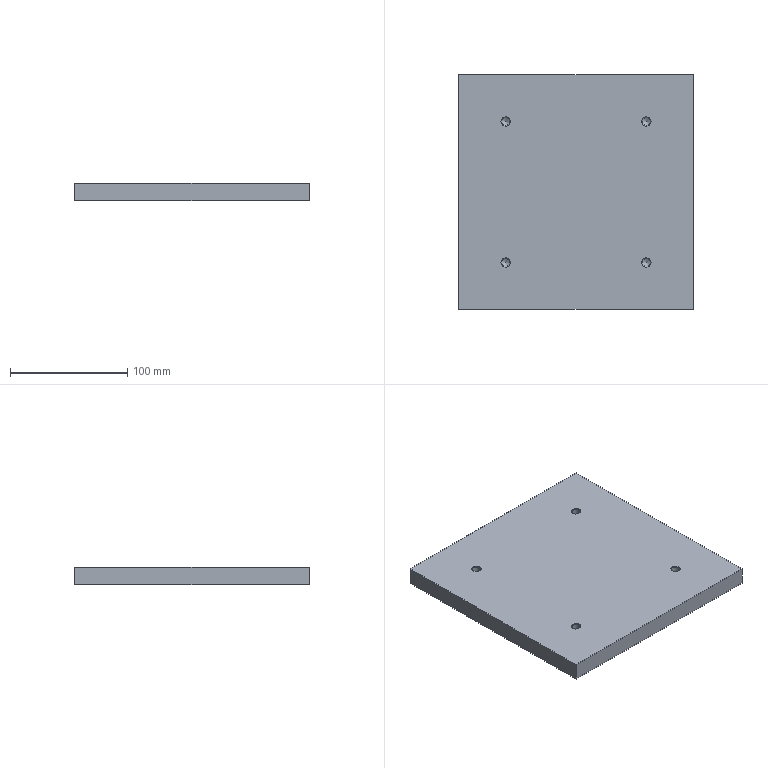Part | NX | features DATUM_CSYS 6, EXTRACT_FACE 6, SKETCH 5, HOLE PACKAGE 4, SIMPLE HOLE 4, SYMBOLIC_THREAD 4, Instance Feature 2, Mirror Feature 2, EXTRUDE 1 | 1 solid | 18 faces | box 200 x 200 x 15 mm | volume 597996 mm3 | cone 8 | plane 6 | cylinder 4 | commonest cylinder face diameters 6.8 x4
STEP:
#1=CARTESIAN_POINT('',(0.,200.,0.));
#2=VERTEX_POINT('',#1);
#3=CARTESIAN_POINT('',(0.,0.,0.));
#4=VERTEX_POINT('',#3);
#5=CARTESIAN_POINT('',(0.,200.,0.));
#6=DIRECTION('',(0.,-1.,0.));
#7=VECTOR('',#6,1000.);
#8=LINE('',#5,#7);
#9=EDGE_CURVE('',#2,#4,#8,.T.);
#10=ORIENTED_EDGE('',*,*,#9,.T.);
#11=CARTESIAN_POINT('',(0.,0.,15.));
#12=VERTEX_POINT('',#11);
#13=CARTESIAN_POINT('',(0.,0.,15.));
#14=DIRECTION('',(0.,0.,-1.));
#15=VECTOR('',#14,1000.);
#16=LINE('',#13,#15);
#17=EDGE_CURVE('',#12,#4,#16,.T.);
#18=ORIENTED_EDGE('',*,*,#17,.F.);
#19=CARTESIAN_POINT('',(0.,200.,15.));
#20=VERTEX_POINT('',#19);
#21=CARTESIAN_POINT('',(0.,200.,15.));
#22=DIRECTION('',(0.,-1.,0.));
#23=VECTOR('',#22,1000.);
#24=LINE('',#21,#23);
#25=EDGE_CURVE('',#20,#12,#24,.T.);
#26=ORIENTED_EDGE('',*,*,#25,.F.);
#27=CARTESIAN_POINT('',(0.,200.,15.));
#28=DIRECTION('',(0.,0.,-1.));
#29=VECTOR('',#28,1000.);
#30=LINE('',#27,#29);
#31=EDGE_CURVE('',#20,#2,#30,.T.);
#32=ORIENTED_EDGE('',*,*,#31,.T.);
#33=EDGE_LOOP('',(#10,#18,#26,#32));
#34=FACE_BOUND('',#33,.T.);
#35=CARTESIAN_POINT('',(0.,200.,15.));
#36=DIRECTION('',(1.,0.,0.));
#37=DIRECTION('',(0.,1.,0.));
#38=AXIS2_PLACEMENT_3D('',#35,#36,#37);
#39=PLANE('',#38);
#40=ADVANCED_FACE('',(#34),#39,.F.);
#41=CARTESIAN_POINT('',(200.,0.,0.));
#42=VERTEX_POINT('',#41);
#43=CARTESIAN_POINT('',(0.,0.,0.));
#44=DIRECTION('',(1.,0.,0.));
#45=VECTOR('',#44,1000.);
#46=LINE('',#43,#45);
#47=EDGE_CURVE('',#4,#42,#46,.T.);
#48=ORIENTED_EDGE('',*,*,#47,.T.);
#49=CARTESIAN_POINT('',(200.,0.,15.));
#50=VERTEX_POINT('',#49);
#51=CARTESIAN_POINT('',(200.,0.,15.));
#52=DIRECTION('',(0.,0.,-1.));
#53=VECTOR('',#52,1000.);
#54=LINE('',#51,#53);
#55=EDGE_CURVE('',#50,#42,#54,.T.);
#56=ORIENTED_EDGE('',*,*,#55,.F.);
#57=CARTESIAN_POINT('',(0.,0.,15.));
#58=DIRECTION('',(1.,0.,0.));
#59=VECTOR('',#58,1000.);
#60=LINE('',#57,#59);
#61=EDGE_CURVE('',#12,#50,#60,.T.);
#62=ORIENTED_EDGE('',*,*,#61,.F.);
#63=ORIENTED_EDGE('',*,*,#17,.T.);
#64=EDGE_LOOP('',(#48,#56,#62,#63));
#65=FACE_BOUND('',#64,.T.);
#66=CARTESIAN_POINT('',(0.,0.,15.));
#67=DIRECTION('',(0.,1.,0.));
#68=DIRECTION('',(0.,0.,1.));
#69=AXIS2_PLACEMENT_3D('',#66,#67,#68);
#70=PLANE('',#69);
#71=ADVANCED_FACE('',(#65),#70,.F.);
#72=CARTESIAN_POINT('',(200.,200.,0.));
#73=VERTEX_POINT('',#72);
#74=CARTESIAN_POINT('',(200.,0.,0.));
#75=DIRECTION('',(0.,1.,0.));
#76=VECTOR('',#75,1000.);
#77=LINE('',#74,#76);
#78=EDGE_CURVE('',#42,#73,#77,.T.);
#79=ORIENTED_EDGE('',*,*,#78,.T.);
#80=CARTESIAN_POINT('',(200.,200.,15.));
#81=VERTEX_POINT('',#80);
#82=CARTESIAN_POINT('',(200.,200.,15.));
#83=DIRECTION('',(0.,0.,-1.));
#84=VECTOR('',#83,1000.);
#85=LINE('',#82,#84);
#86=EDGE_CURVE('',#81,#73,#85,.T.);
#87=ORIENTED_EDGE('',*,*,#86,.F.);
#88=CARTESIAN_POINT('',(200.,0.,15.));
#89=DIRECTION('',(0.,1.,0.));
#90=VECTOR('',#89,1000.);
#91=LINE('',#88,#90);
#92=EDGE_CURVE('',#50,#81,#91,.T.);
#93=ORIENTED_EDGE('',*,*,#92,.F.);
#94=ORIENTED_EDGE('',*,*,#55,.T.);
#95=EDGE_LOOP('',(#79,#87,#93,#94));
#96=FACE_BOUND('',#95,.T.);
#97=CARTESIAN_POINT('',(200.,0.,15.));
#98=DIRECTION('',(-1.,0.,0.));
#99=DIRECTION('',(0.,-1.,0.));
#100=AXIS2_PLACEMENT_3D('',#97,#98,#99);
#101=PLANE('',#100);
#102=ADVANCED_FACE('',(#96),#101,.F.);
#103=CARTESIAN_POINT('',(200.,200.,0.));
#104=DIRECTION('',(-1.,0.,0.));
#105=VECTOR('',#104,1000.);
#106=LINE('',#103,#105);
#107=EDGE_CURVE('',#73,#2,#106,.T.);
#108=ORIENTED_EDGE('',*,*,#107,.T.);
#109=ORIENTED_EDGE('',*,*,#31,.F.);
#110=CARTESIAN_POINT('',(200.,200.,15.));
#111=DIRECTION('',(-1.,0.,0.));
#112=VECTOR('',#111,1000.);
#113=LINE('',#110,#112);
#114=EDGE_CURVE('',#81,#20,#113,.T.);
#115=ORIENTED_EDGE('',*,*,#114,.F.);
#116=ORIENTED_EDGE('',*,*,#86,.T.);
#117=EDGE_LOOP('',(#108,#109,#115,#116));
#118=FACE_BOUND('',#117,.T.);
#119=CARTESIAN_POINT('',(200.,200.,15.));
#120=DIRECTION('',(0.,-1.,0.));
#121=DIRECTION('',(1.,0.,0.));
#122=AXIS2_PLACEMENT_3D('',#119,#120,#121);
#123=PLANE('',#122);
#124=ADVANCED_FACE('',(#118),#123,.F.);
#125=CARTESIAN_POINT('',(44.,160.,15.));
#126=VERTEX_POINT('',#125);
#127=CARTESIAN_POINT('',(40.,160.,15.));
#128=DIRECTION('',(0.,0.,1.));
#129=DIRECTION('',(1.,0.,0.));
#130=AXIS2_PLACEMENT_3D('',#127,#128,#129);
#131=CIRCLE('',#130,4.);
#132=EDGE_CURVE('',#126,#126,#131,.F.);
#133=ORIENTED_EDGE('',*,*,#132,.T.);
#134=EDGE_LOOP('',(#133));
#135=FACE_BOUND('',#134,.T.);
#136=CARTESIAN_POINT('',(44.,40.,15.));
#137=VERTEX_POINT('',#136);
#138=CARTESIAN_POINT('',(40.,40.,15.));
#139=DIRECTION('',(0.,0.,1.));
#140=DIRECTION('',(1.,0.,0.));
#141=AXIS2_PLACEMENT_3D('',#138,#139,#140);
#142=CIRCLE('',#141,4.);
#143=EDGE_CURVE('',#137,#137,#142,.F.);
#144=ORIENTED_EDGE('',*,*,#143,.T.);
#145=EDGE_LOOP('',(#144));
#146=FACE_BOUND('',#145,.T.);
#147=CARTESIAN_POINT('',(164.,160.,15.));
#148=VERTEX_POINT('',#147);
#149=CARTESIAN_POINT('',(160.,160.,15.));
#150=DIRECTION('',(0.,0.,1.));
#151=DIRECTION('',(1.,0.,0.));
#152=AXIS2_PLACEMENT_3D('',#149,#150,#151);
#153=CIRCLE('',#152,4.);
#154=EDGE_CURVE('',#148,#148,#153,.F.);
#155=ORIENTED_EDGE('',*,*,#154,.T.);
#156=EDGE_LOOP('',(#155));
#157=FACE_BOUND('',#156,.T.);
#158=CARTESIAN_POINT('',(164.,40.,15.));
#159=VERTEX_POINT('',#158);
#160=CARTESIAN_POINT('',(160.,40.,15.));
#161=DIRECTION('',(0.,0.,1.));
#162=DIRECTION('',(1.,0.,0.));
#163=AXIS2_PLACEMENT_3D('',#160,#161,#162);
#164=CIRCLE('',#163,4.);
#165=EDGE_CURVE('',#159,#159,#164,.F.);
#166=ORIENTED_EDGE('',*,*,#165,.T.);
#167=EDGE_LOOP('',(#166));
#168=FACE_BOUND('',#167,.T.);
#169=ORIENTED_EDGE('',*,*,#25,.T.);
#170=ORIENTED_EDGE('',*,*,#61,.T.);
#171=ORIENTED_EDGE('',*,*,#92,.T.);
#172=ORIENTED_EDGE('',*,*,#114,.T.);
#173=EDGE_LOOP('',(#169,#170,#171,#172));
#174=FACE_BOUND('',#173,.T.);
#175=CARTESIAN_POINT('',(0.,0.,15.));
#176=DIRECTION('',(0.,0.,1.));
#177=DIRECTION('',(1.,0.,0.));
#178=AXIS2_PLACEMENT_3D('',#175,#176,#177);
#179=PLANE('',#178);
#180=ADVANCED_FACE('',(#135,#146,#157,#168,#174),#179,.T.);
#181=CARTESIAN_POINT('',(40.071,160.,0.));
#182=VERTEX_POINT('',#181);
#183=CARTESIAN_POINT('',(40.,160.,0.));
#184=DIRECTION('',(0.,0.,1.));
#185=DIRECTION('',(1.,0.,0.));
#186=AXIS2_PLACEMENT_3D('',#183,#184,#185);
#187=CIRCLE('',#186,0.07144);
#188=EDGE_CURVE('',#182,#182,#187,.T.);
#189=ORIENTED_EDGE('',*,*,#188,.T.);
#190=EDGE_LOOP('',(#189));
#191=FACE_BOUND('',#190,.T.);
#192=CARTESIAN_POINT('',(40.071,40.,0.));
#193=VERTEX_POINT('',#192);
#194=CARTESIAN_POINT('',(40.,40.,0.));
#195=DIRECTION('',(0.,0.,1.));
#196=DIRECTION('',(1.,0.,0.));
#197=AXIS2_PLACEMENT_3D('',#194,#195,#196);
#198=CIRCLE('',#197,0.07144);
#199=EDGE_CURVE('',#193,#193,#198,.T.);
#200=ORIENTED_EDGE('',*,*,#199,.T.);
#201=EDGE_LOOP('',(#200));
#202=FACE_BOUND('',#201,.T.);
#203=CARTESIAN_POINT('',(160.071,160.,0.));
#204=VERTEX_POINT('',#203);
#205=CARTESIAN_POINT('',(160.,160.,0.));
#206=DIRECTION('',(0.,0.,1.));
#207=DIRECTION('',(1.,0.,0.));
#208=AXIS2_PLACEMENT_3D('',#205,#206,#207);
#209=CIRCLE('',#208,0.07144);
#210=EDGE_CURVE('',#204,#204,#209,.T.);
#211=ORIENTED_EDGE('',*,*,#210,.T.);
#212=EDGE_LOOP('',(#211));
#213=FACE_BOUND('',#212,.T.);
#214=CARTESIAN_POINT('',(160.071,40.,0.));
#215=VERTEX_POINT('',#214);
#216=CARTESIAN_POINT('',(160.,40.,0.));
#217=DIRECTION('',(0.,0.,1.));
#218=DIRECTION('',(1.,0.,0.));
#219=AXIS2_PLACEMENT_3D('',#216,#217,#218);
#220=CIRCLE('',#219,0.07144);
#221=EDGE_CURVE('',#215,#215,#220,.T.);
#222=ORIENTED_EDGE('',*,*,#221,.T.);
#223=EDGE_LOOP('',(#222));
#224=FACE_BOUND('',#223,.T.);
#225=ORIENTED_EDGE('',*,*,#9,.F.);
#226=ORIENTED_EDGE('',*,*,#107,.F.);
#227=ORIENTED_EDGE('',*,*,#78,.F.);
#228=ORIENTED_EDGE('',*,*,#47,.F.);
#229=EDGE_LOOP('',(#225,#226,#227,#228));
#230=FACE_BOUND('',#229,.T.);
#231=CARTESIAN_POINT('',(0.,0.,0.));
#232=DIRECTION('',(0.,0.,1.));
#233=DIRECTION('',(1.,0.,0.));
#234=AXIS2_PLACEMENT_3D('',#231,#232,#233);
#235=PLANE('',#234);
#236=ADVANCED_FACE('',(#191,#202,#213,#224,#230),#235,.F.);
#237=CARTESIAN_POINT('',(156.6,40.,2.));
#238=VERTEX_POINT('',#237);
#239=CARTESIAN_POINT('',(160.,40.,2.));
#240=DIRECTION('',(0.,0.,-1.));
#241=DIRECTION('',(-1.,0.,0.));
#242=AXIS2_PLACEMENT_3D('',#239,#240,#241);
#243=CIRCLE('',#242,3.4);
#244=EDGE_CURVE('',#238,#238,#243,.F.);
#245=ORIENTED_EDGE('',*,*,#244,.T.);
#246=EDGE_LOOP('',(#245));
#247=FACE_BOUND('',#246,.T.);
#248=ORIENTED_EDGE('',*,*,#221,.F.);
#249=EDGE_LOOP('',(#248));
#250=FACE_BOUND('',#249,.T.);
#251=CARTESIAN_POINT('',(160.,40.,2.));
#252=DIRECTION('',(0.,0.,1.));
#253=DIRECTION('',(1.,0.,0.));
#254=AXIS2_PLACEMENT_3D('',#251,#252,#253);
#255=CONICAL_SURFACE('',#254,3.4,1.03);
#256=ADVANCED_FACE('',(#247,#250),#255,.F.);
#257=CARTESIAN_POINT('',(163.4,40.,14.4));
#258=VERTEX_POINT('',#257);
#259=CARTESIAN_POINT('',(160.,40.,14.4));
#260=DIRECTION('',(0.,0.,1.));
#261=DIRECTION('',(1.,0.,0.));
#262=AXIS2_PLACEMENT_3D('',#259,#260,#261);
#263=CIRCLE('',#262,3.4);
#264=EDGE_CURVE('',#258,#258,#263,.T.);
#265=ORIENTED_EDGE('',*,*,#264,.T.);
#266=EDGE_LOOP('',(#265));
#267=FACE_BOUND('',#266,.T.);
#268=ORIENTED_EDGE('',*,*,#244,.F.);
#269=EDGE_LOOP('',(#268));
#270=FACE_BOUND('',#269,.T.);
#271=CARTESIAN_POINT('',(160.,40.,15.));
#272=DIRECTION('',(0.,0.,-1.));
#273=DIRECTION('',(-1.,0.,0.));
#274=AXIS2_PLACEMENT_3D('',#271,#272,#273);
#275=CYLINDRICAL_SURFACE('',#274,3.4);
#276=ADVANCED_FACE('',(#267,#270),#275,.F.);
#277=ORIENTED_EDGE('',*,*,#264,.F.);
#278=EDGE_LOOP('',(#277));
#279=FACE_BOUND('',#278,.T.);
#280=ORIENTED_EDGE('',*,*,#165,.F.);
#281=EDGE_LOOP('',(#280));
#282=FACE_BOUND('',#281,.T.);
#283=CARTESIAN_POINT('',(160.,40.,15.));
#284=DIRECTION('',(0.,0.,1.));
#285=DIRECTION('',(1.,0.,0.));
#286=AXIS2_PLACEMENT_3D('',#283,#284,#285);
#287=CONICAL_SURFACE('',#286,4.,0.7854);
#288=ADVANCED_FACE('',(#279,#282),#287,.F.);
#289=CARTESIAN_POINT('',(156.6,160.,2.));
#290=VERTEX_POINT('',#289);
#291=CARTESIAN_POINT('',(160.,160.,2.));
#292=DIRECTION('',(0.,0.,-1.));
#293=DIRECTION('',(-1.,0.,0.));
#294=AXIS2_PLACEMENT_3D('',#291,#292,#293);
#295=CIRCLE('',#294,3.4);
#296=EDGE_CURVE('',#290,#290,#295,.T.);
#297=ORIENTED_EDGE('',*,*,#296,.F.);
#298=EDGE_LOOP('',(#297));
#299=FACE_BOUND('',#298,.T.);
#300=ORIENTED_EDGE('',*,*,#210,.F.);
#301=EDGE_LOOP('',(#300));
#302=FACE_BOUND('',#301,.T.);
#303=CARTESIAN_POINT('',(160.,160.,2.));
#304=DIRECTION('',(0.,0.,1.));
#305=DIRECTION('',(1.,0.,0.));
#306=AXIS2_PLACEMENT_3D('',#303,#304,#305);
#307=CONICAL_SURFACE('',#306,3.4,1.03);
#308=ADVANCED_FACE('',(#299,#302),#307,.F.);
#309=CARTESIAN_POINT('',(163.4,160.,14.4));
#310=VERTEX_POINT('',#309);
#311=CARTESIAN_POINT('',(160.,160.,14.4));
#312=DIRECTION('',(0.,0.,1.));
#313=DIRECTION('',(1.,0.,0.));
#314=AXIS2_PLACEMENT_3D('',#311,#312,#313);
#315=CIRCLE('',#314,3.4);
#316=EDGE_CURVE('',#310,#310,#315,.F.);
#317=ORIENTED_EDGE('',*,*,#316,.F.);
#318=EDGE_LOOP('',(#317));
#319=FACE_BOUND('',#318,.T.);
#320=ORIENTED_EDGE('',*,*,#296,.T.);
#321=EDGE_LOOP('',(#320));
#322=FACE_BOUND('',#321,.T.);
#323=CARTESIAN_POINT('',(160.,160.,15.));
#324=DIRECTION('',(0.,0.,-1.));
#325=DIRECTION('',(-1.,0.,0.));
#326=AXIS2_PLACEMENT_3D('',#323,#324,#325);
#327=CYLINDRICAL_SURFACE('',#326,3.4);
#328=ADVANCED_FACE('',(#319,#322),#327,.F.);
#329=ORIENTED_EDGE('',*,*,#154,.F.);
#330=EDGE_LOOP('',(#329));
#331=FACE_BOUND('',#330,.T.);
#332=ORIENTED_EDGE('',*,*,#316,.T.);
#333=EDGE_LOOP('',(#332));
#334=FACE_BOUND('',#333,.T.);
#335=CARTESIAN_POINT('',(160.,160.,14.4));
#336=DIRECTION('',(0.,0.,1.));
#337=DIRECTION('',(1.,0.,0.));
#338=AXIS2_PLACEMENT_3D('',#335,#336,#337);
#339=CONICAL_SURFACE('',#338,3.4,0.7854);
#340=ADVANCED_FACE('',(#331,#334),#339,.F.);
#341=CARTESIAN_POINT('',(36.6,40.,2.));
#342=VERTEX_POINT('',#341);
#343=CARTESIAN_POINT('',(40.,40.,2.));
#344=DIRECTION('',(0.,0.,-1.));
#345=DIRECTION('',(-1.,0.,0.));
#346=AXIS2_PLACEMENT_3D('',#343,#344,#345);
#347=CIRCLE('',#346,3.4);
#348=EDGE_CURVE('',#342,#342,#347,.T.);
#349=ORIENTED_EDGE('',*,*,#348,.F.);
#350=EDGE_LOOP('',(#349));
#351=FACE_BOUND('',#350,.T.);
#352=ORIENTED_EDGE('',*,*,#199,.F.);
#353=EDGE_LOOP('',(#352));
#354=FACE_BOUND('',#353,.T.);
#355=CARTESIAN_POINT('',(40.,40.,2.));
#356=DIRECTION('',(0.,0.,1.));
#357=DIRECTION('',(1.,0.,0.));
#358=AXIS2_PLACEMENT_3D('',#355,#356,#357);
#359=CONICAL_SURFACE('',#358,3.4,1.03);
#360=ADVANCED_FACE('',(#351,#354),#359,.F.);
#361=CARTESIAN_POINT('',(43.4,40.,14.4));
#362=VERTEX_POINT('',#361);
#363=CARTESIAN_POINT('',(40.,40.,14.4));
#364=DIRECTION('',(0.,0.,1.));
#365=DIRECTION('',(1.,0.,0.));
#366=AXIS2_PLACEMENT_3D('',#363,#364,#365);
#367=CIRCLE('',#366,3.4);
#368=EDGE_CURVE('',#362,#362,#367,.F.);
#369=ORIENTED_EDGE('',*,*,#368,.F.);
#370=EDGE_LOOP('',(#369));
#371=FACE_BOUND('',#370,.T.);
#372=ORIENTED_EDGE('',*,*,#348,.T.);
#373=EDGE_LOOP('',(#372));
#374=FACE_BOUND('',#373,.T.);
#375=CARTESIAN_POINT('',(40.,40.,15.));
#376=DIRECTION('',(0.,0.,-1.));
#377=DIRECTION('',(-1.,0.,0.));
#378=AXIS2_PLACEMENT_3D('',#375,#376,#377);
#379=CYLINDRICAL_SURFACE('',#378,3.4);
#380=ADVANCED_FACE('',(#371,#374),#379,.F.);
#381=ORIENTED_EDGE('',*,*,#368,.T.);
#382=EDGE_LOOP('',(#381));
#383=FACE_BOUND('',#382,.T.);
#384=ORIENTED_EDGE('',*,*,#143,.F.);
#385=EDGE_LOOP('',(#384));
#386=FACE_BOUND('',#385,.T.);
#387=CARTESIAN_POINT('',(40.,40.,15.));
#388=DIRECTION('',(0.,0.,1.));
#389=DIRECTION('',(1.,0.,0.));
#390=AXIS2_PLACEMENT_3D('',#387,#388,#389);
#391=CONICAL_SURFACE('',#390,4.,0.7854);
#392=ADVANCED_FACE('',(#383,#386),#391,.F.);
#393=CARTESIAN_POINT('',(36.6,160.,2.));
#394=VERTEX_POINT('',#393);
#395=CARTESIAN_POINT('',(40.,160.,2.));
#396=DIRECTION('',(0.,0.,-1.));
#397=DIRECTION('',(-1.,0.,0.));
#398=AXIS2_PLACEMENT_3D('',#395,#396,#397);
#399=CIRCLE('',#398,3.4);
#400=EDGE_CURVE('',#394,#394,#399,.F.);
#401=ORIENTED_EDGE('',*,*,#400,.T.);
#402=EDGE_LOOP('',(#401));
#403=FACE_BOUND('',#402,.T.);
#404=ORIENTED_EDGE('',*,*,#188,.F.);
#405=EDGE_LOOP('',(#404));
#406=FACE_BOUND('',#405,.T.);
#407=CARTESIAN_POINT('',(40.,160.,2.));
#408=DIRECTION('',(0.,0.,1.));
#409=DIRECTION('',(1.,0.,0.));
#410=AXIS2_PLACEMENT_3D('',#407,#408,#409);
#411=CONICAL_SURFACE('',#410,3.4,1.03);
#412=ADVANCED_FACE('',(#403,#406),#411,.F.);
#413=CARTESIAN_POINT('',(43.4,160.,14.4));
#414=VERTEX_POINT('',#413);
#415=CARTESIAN_POINT('',(40.,160.,14.4));
#416=DIRECTION('',(0.,0.,1.));
#417=DIRECTION('',(1.,0.,0.));
#418=AXIS2_PLACEMENT_3D('',#415,#416,#417);
#419=CIRCLE('',#418,3.4);
#420=EDGE_CURVE('',#414,#414,#419,.T.);
#421=ORIENTED_EDGE('',*,*,#420,.T.);
#422=EDGE_LOOP('',(#421));
#423=FACE_BOUND('',#422,.T.);
#424=ORIENTED_EDGE('',*,*,#400,.F.);
#425=EDGE_LOOP('',(#424));
#426=FACE_BOUND('',#425,.T.);
#427=CARTESIAN_POINT('',(40.,160.,15.));
#428=DIRECTION('',(0.,0.,-1.));
#429=DIRECTION('',(-1.,0.,0.));
#430=AXIS2_PLACEMENT_3D('',#427,#428,#429);
#431=CYLINDRICAL_SURFACE('',#430,3.4);
#432=ADVANCED_FACE('',(#423,#426),#431,.F.);
#433=ORIENTED_EDGE('',*,*,#420,.F.);
#434=EDGE_LOOP('',(#433));
#435=FACE_BOUND('',#434,.T.);
#436=ORIENTED_EDGE('',*,*,#132,.F.);
#437=EDGE_LOOP('',(#436));
#438=FACE_BOUND('',#437,.T.);
#439=CARTESIAN_POINT('',(40.,160.,15.));
#440=DIRECTION('',(0.,0.,1.));
#441=DIRECTION('',(1.,0.,0.));
#442=AXIS2_PLACEMENT_3D('',#439,#440,#441);
#443=CONICAL_SURFACE('',#442,4.,0.7854);
#444=ADVANCED_FACE('',(#435,#438),#443,.F.);
#445=CLOSED_SHELL('',(#40,#71,#102,#124,#180,#236,#256,#276,#288,#308,#328,#340,#360,#380,#392,#412,#432,#444));
#446=MANIFOLD_SOLID_BREP('',#445);
#447=(LENGTH_UNIT()NAMED_UNIT(*)SI_UNIT(.MILLI.,.METRE.));
#448=UNCERTAINTY_MEASURE_WITH_UNIT(LENGTH_MEASURE(0.00001),#447,'','');
#449=(NAMED_UNIT(*)PLANE_ANGLE_UNIT()SI_UNIT($,.RADIAN.));
#450=(NAMED_UNIT(*)SI_UNIT($,.STERADIAN.)SOLID_ANGLE_UNIT());
#451=(GEOMETRIC_REPRESENTATION_CONTEXT(3)GLOBAL_UNCERTAINTY_ASSIGNED_CONTEXT((#448))GLOBAL_UNIT_ASSIGNED_CONTEXT((#447,#449,#450))REPRESENTATION_CONTEXT('',''));
#452=ADVANCED_BREP_SHAPE_REPRESENTATION('',(#446),#451);